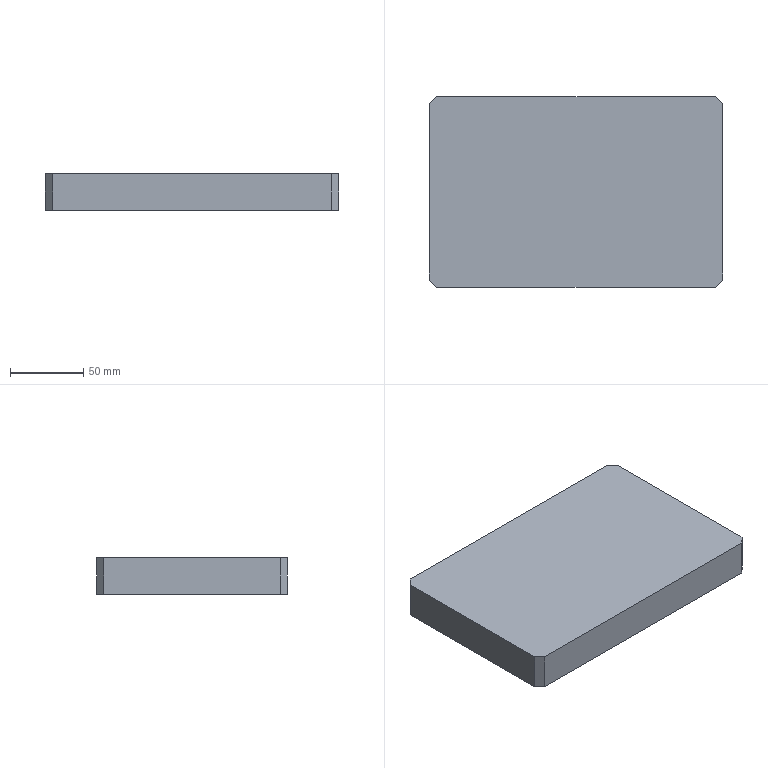Part | SolidWorks | features Chamfer 1, Extrusion 1 | 1 solid | 10 faces | box 200 x 130 x 25 mm | volume 648750 mm3 | plane 10
STEP:
#1=CARTESIAN_POINT('',(100.,-60.,25.));
#2=VERTEX_POINT('',#1);
#3=CARTESIAN_POINT('',(100.,60.,25.));
#4=VERTEX_POINT('',#3);
#5=CARTESIAN_POINT('',(100.,65.,25.));
#6=DIRECTION('',(0.,1.,0.));
#7=VECTOR('',#6,1000.);
#8=LINE('',#5,#7);
#9=EDGE_CURVE('',#2,#4,#8,.T.);
#10=ORIENTED_EDGE('',*,*,#9,.F.);
#11=CARTESIAN_POINT('',(100.,-60.,0.));
#12=VERTEX_POINT('',#11);
#13=CARTESIAN_POINT('',(100.,-60.,25.));
#14=DIRECTION('',(0.,0.,-1.));
#15=VECTOR('',#14,1000.);
#16=LINE('',#13,#15);
#17=EDGE_CURVE('',#2,#12,#16,.T.);
#18=ORIENTED_EDGE('',*,*,#17,.T.);
#19=CARTESIAN_POINT('',(100.,60.,0.));
#20=VERTEX_POINT('',#19);
#21=CARTESIAN_POINT('',(100.,65.,0.));
#22=DIRECTION('',(0.,1.,0.));
#23=VECTOR('',#22,1000.);
#24=LINE('',#21,#23);
#25=EDGE_CURVE('',#12,#20,#24,.T.);
#26=ORIENTED_EDGE('',*,*,#25,.T.);
#27=CARTESIAN_POINT('',(100.,60.,25.));
#28=DIRECTION('',(0.,0.,1.));
#29=VECTOR('',#28,1000.);
#30=LINE('',#27,#29);
#31=EDGE_CURVE('',#20,#4,#30,.T.);
#32=ORIENTED_EDGE('',*,*,#31,.T.);
#33=EDGE_LOOP('',(#10,#18,#26,#32));
#34=FACE_OUTER_BOUND('',#33,.T.);
#35=CARTESIAN_POINT('',(100.,65.,25.));
#36=DIRECTION('',(-1.,0.,0.));
#37=DIRECTION('',(0.,-1.,0.));
#38=AXIS2_PLACEMENT_3D('',#35,#36,#37);
#39=PLANE('',#38);
#40=ADVANCED_FACE('',(#34),#39,.F.);
#41=CARTESIAN_POINT('',(95.,65.,0.));
#42=VERTEX_POINT('',#41);
#43=CARTESIAN_POINT('',(-95.,65.,0.));
#44=VERTEX_POINT('',#43);
#45=CARTESIAN_POINT('',(-100.,65.,0.));
#46=DIRECTION('',(-1.,0.,0.));
#47=VECTOR('',#46,1000.);
#48=LINE('',#45,#47);
#49=EDGE_CURVE('',#42,#44,#48,.T.);
#50=ORIENTED_EDGE('',*,*,#49,.T.);
#51=CARTESIAN_POINT('',(-95.,65.,25.));
#52=VERTEX_POINT('',#51);
#53=CARTESIAN_POINT('',(-95.,65.,25.));
#54=DIRECTION('',(0.,0.,1.));
#55=VECTOR('',#54,1000.);
#56=LINE('',#53,#55);
#57=EDGE_CURVE('',#44,#52,#56,.T.);
#58=ORIENTED_EDGE('',*,*,#57,.T.);
#59=CARTESIAN_POINT('',(95.,65.,25.));
#60=VERTEX_POINT('',#59);
#61=CARTESIAN_POINT('',(-100.,65.,25.));
#62=DIRECTION('',(-1.,0.,0.));
#63=VECTOR('',#62,1000.);
#64=LINE('',#61,#63);
#65=EDGE_CURVE('',#60,#52,#64,.T.);
#66=ORIENTED_EDGE('',*,*,#65,.F.);
#67=CARTESIAN_POINT('',(95.,65.,25.));
#68=DIRECTION('',(0.,0.,-1.));
#69=VECTOR('',#68,1000.);
#70=LINE('',#67,#69);
#71=EDGE_CURVE('',#60,#42,#70,.T.);
#72=ORIENTED_EDGE('',*,*,#71,.T.);
#73=EDGE_LOOP('',(#50,#58,#66,#72));
#74=FACE_OUTER_BOUND('',#73,.T.);
#75=CARTESIAN_POINT('',(-100.,65.,25.));
#76=DIRECTION('',(0.,-1.,0.));
#77=DIRECTION('',(0.,0.,-1.));
#78=AXIS2_PLACEMENT_3D('',#75,#76,#77);
#79=PLANE('',#78);
#80=ADVANCED_FACE('',(#74),#79,.F.);
#81=CARTESIAN_POINT('',(-100.,60.,0.));
#82=VERTEX_POINT('',#81);
#83=CARTESIAN_POINT('',(-100.,-60.,0.));
#84=VERTEX_POINT('',#83);
#85=CARTESIAN_POINT('',(-100.,65.,0.));
#86=DIRECTION('',(0.,-1.,0.));
#87=VECTOR('',#86,1000.);
#88=LINE('',#85,#87);
#89=EDGE_CURVE('',#82,#84,#88,.T.);
#90=ORIENTED_EDGE('',*,*,#89,.T.);
#91=CARTESIAN_POINT('',(-100.,-60.,25.));
#92=VERTEX_POINT('',#91);
#93=CARTESIAN_POINT('',(-100.,-60.,25.));
#94=DIRECTION('',(0.,0.,1.));
#95=VECTOR('',#94,1000.);
#96=LINE('',#93,#95);
#97=EDGE_CURVE('',#84,#92,#96,.T.);
#98=ORIENTED_EDGE('',*,*,#97,.T.);
#99=CARTESIAN_POINT('',(-100.,60.,25.));
#100=VERTEX_POINT('',#99);
#101=CARTESIAN_POINT('',(-100.,65.,25.));
#102=DIRECTION('',(0.,-1.,0.));
#103=VECTOR('',#102,1000.);
#104=LINE('',#101,#103);
#105=EDGE_CURVE('',#100,#92,#104,.T.);
#106=ORIENTED_EDGE('',*,*,#105,.F.);
#107=CARTESIAN_POINT('',(-100.,60.,25.));
#108=DIRECTION('',(0.,0.,-1.));
#109=VECTOR('',#108,1000.);
#110=LINE('',#107,#109);
#111=EDGE_CURVE('',#100,#82,#110,.T.);
#112=ORIENTED_EDGE('',*,*,#111,.T.);
#113=EDGE_LOOP('',(#90,#98,#106,#112));
#114=FACE_OUTER_BOUND('',#113,.T.);
#115=CARTESIAN_POINT('',(-100.,65.,25.));
#116=DIRECTION('',(1.,0.,0.));
#117=DIRECTION('',(0.,1.,0.));
#118=AXIS2_PLACEMENT_3D('',#115,#116,#117);
#119=PLANE('',#118);
#120=ADVANCED_FACE('',(#114),#119,.F.);
#121=CARTESIAN_POINT('',(-95.,-65.,25.));
#122=VERTEX_POINT('',#121);
#123=CARTESIAN_POINT('',(95.,-65.,25.));
#124=VERTEX_POINT('',#123);
#125=CARTESIAN_POINT('',(-100.,-65.,25.));
#126=DIRECTION('',(1.,0.,0.));
#127=VECTOR('',#126,1000.);
#128=LINE('',#125,#127);
#129=EDGE_CURVE('',#122,#124,#128,.T.);
#130=ORIENTED_EDGE('',*,*,#129,.F.);
#131=CARTESIAN_POINT('',(-95.,-65.,0.));
#132=VERTEX_POINT('',#131);
#133=CARTESIAN_POINT('',(-95.,-65.,25.));
#134=DIRECTION('',(0.,0.,-1.));
#135=VECTOR('',#134,1000.);
#136=LINE('',#133,#135);
#137=EDGE_CURVE('',#122,#132,#136,.T.);
#138=ORIENTED_EDGE('',*,*,#137,.T.);
#139=CARTESIAN_POINT('',(95.,-65.,0.));
#140=VERTEX_POINT('',#139);
#141=CARTESIAN_POINT('',(-100.,-65.,0.));
#142=DIRECTION('',(1.,0.,0.));
#143=VECTOR('',#142,1000.);
#144=LINE('',#141,#143);
#145=EDGE_CURVE('',#132,#140,#144,.T.);
#146=ORIENTED_EDGE('',*,*,#145,.T.);
#147=CARTESIAN_POINT('',(95.,-65.,25.));
#148=DIRECTION('',(0.,0.,1.));
#149=VECTOR('',#148,1000.);
#150=LINE('',#147,#149);
#151=EDGE_CURVE('',#140,#124,#150,.T.);
#152=ORIENTED_EDGE('',*,*,#151,.T.);
#153=EDGE_LOOP('',(#130,#138,#146,#152));
#154=FACE_OUTER_BOUND('',#153,.T.);
#155=CARTESIAN_POINT('',(-100.,-65.,25.));
#156=DIRECTION('',(0.,1.,0.));
#157=DIRECTION('',(0.,0.,1.));
#158=AXIS2_PLACEMENT_3D('',#155,#156,#157);
#159=PLANE('',#158);
#160=ADVANCED_FACE('',(#154),#159,.F.);
#161=ORIENTED_EDGE('',*,*,#105,.T.);
#162=CARTESIAN_POINT('',(-80.,-80.,25.));
#163=DIRECTION('',(0.7071,-0.7071,0.));
#164=VECTOR('',#163,1000.);
#165=LINE('',#162,#164);
#166=EDGE_CURVE('',#92,#122,#165,.T.);
#167=ORIENTED_EDGE('',*,*,#166,.T.);
#168=ORIENTED_EDGE('',*,*,#129,.T.);
#169=CARTESIAN_POINT('',(80.,-80.,25.));
#170=DIRECTION('',(0.7071,0.7071,0.));
#171=VECTOR('',#170,1000.);
#172=LINE('',#169,#171);
#173=EDGE_CURVE('',#124,#2,#172,.T.);
#174=ORIENTED_EDGE('',*,*,#173,.T.);
#175=ORIENTED_EDGE('',*,*,#9,.T.);
#176=CARTESIAN_POINT('',(80.,80.,25.));
#177=DIRECTION('',(-0.7071,0.7071,0.));
#178=VECTOR('',#177,1000.);
#179=LINE('',#176,#178);
#180=EDGE_CURVE('',#4,#60,#179,.T.);
#181=ORIENTED_EDGE('',*,*,#180,.T.);
#182=ORIENTED_EDGE('',*,*,#65,.T.);
#183=CARTESIAN_POINT('',(-80.,80.,25.));
#184=DIRECTION('',(-0.7071,-0.7071,0.));
#185=VECTOR('',#184,1000.);
#186=LINE('',#183,#185);
#187=EDGE_CURVE('',#52,#100,#186,.T.);
#188=ORIENTED_EDGE('',*,*,#187,.T.);
#189=EDGE_LOOP('',(#161,#167,#168,#174,#175,#181,#182,#188));
#190=FACE_OUTER_BOUND('',#189,.T.);
#191=CARTESIAN_POINT('',(0.,0.,25.));
#192=DIRECTION('',(0.,0.,1.));
#193=DIRECTION('',(1.,0.,0.));
#194=AXIS2_PLACEMENT_3D('',#191,#192,#193);
#195=PLANE('',#194);
#196=ADVANCED_FACE('',(#190),#195,.T.);
#197=ORIENTED_EDGE('',*,*,#145,.F.);
#198=CARTESIAN_POINT('',(-95.,-65.,0.));
#199=DIRECTION('',(-0.7071,0.7071,0.));
#200=VECTOR('',#199,1000.);
#201=LINE('',#198,#200);
#202=EDGE_CURVE('',#132,#84,#201,.T.);
#203=ORIENTED_EDGE('',*,*,#202,.T.);
#204=ORIENTED_EDGE('',*,*,#89,.F.);
#205=CARTESIAN_POINT('',(-100.,60.,0.));
#206=DIRECTION('',(0.7071,0.7071,0.));
#207=VECTOR('',#206,1000.);
#208=LINE('',#205,#207);
#209=EDGE_CURVE('',#82,#44,#208,.T.);
#210=ORIENTED_EDGE('',*,*,#209,.T.);
#211=ORIENTED_EDGE('',*,*,#49,.F.);
#212=CARTESIAN_POINT('',(95.,65.,0.));
#213=DIRECTION('',(0.7071,-0.7071,0.));
#214=VECTOR('',#213,1000.);
#215=LINE('',#212,#214);
#216=EDGE_CURVE('',#42,#20,#215,.T.);
#217=ORIENTED_EDGE('',*,*,#216,.T.);
#218=ORIENTED_EDGE('',*,*,#25,.F.);
#219=CARTESIAN_POINT('',(100.,-60.,0.));
#220=DIRECTION('',(-0.7071,-0.7071,0.));
#221=VECTOR('',#220,1000.);
#222=LINE('',#219,#221);
#223=EDGE_CURVE('',#12,#140,#222,.T.);
#224=ORIENTED_EDGE('',*,*,#223,.T.);
#225=EDGE_LOOP('',(#197,#203,#204,#210,#211,#217,#218,#224));
#226=FACE_OUTER_BOUND('',#225,.T.);
#227=CARTESIAN_POINT('',(0.,0.,0.));
#228=DIRECTION('',(0.,0.,1.));
#229=DIRECTION('',(1.,0.,0.));
#230=AXIS2_PLACEMENT_3D('',#227,#228,#229);
#231=PLANE('',#230);
#232=ADVANCED_FACE('',(#226),#231,.F.);
#233=ORIENTED_EDGE('',*,*,#166,.F.);
#234=ORIENTED_EDGE('',*,*,#97,.F.);
#235=ORIENTED_EDGE('',*,*,#202,.F.);
#236=ORIENTED_EDGE('',*,*,#137,.F.);
#237=EDGE_LOOP('',(#233,#234,#235,#236));
#238=FACE_OUTER_BOUND('',#237,.T.);
#239=CARTESIAN_POINT('',(-95.,-65.,25.));
#240=DIRECTION('',(0.7071,0.7071,0.));
#241=DIRECTION('',(0.,0.,-1.));
#242=AXIS2_PLACEMENT_3D('',#239,#240,#241);
#243=PLANE('',#242);
#244=ADVANCED_FACE('',(#238),#243,.F.);
#245=ORIENTED_EDGE('',*,*,#173,.F.);
#246=ORIENTED_EDGE('',*,*,#151,.F.);
#247=ORIENTED_EDGE('',*,*,#223,.F.);
#248=ORIENTED_EDGE('',*,*,#17,.F.);
#249=EDGE_LOOP('',(#245,#246,#247,#248));
#250=FACE_OUTER_BOUND('',#249,.T.);
#251=CARTESIAN_POINT('',(100.,-60.,25.));
#252=DIRECTION('',(-0.7071,0.7071,0.));
#253=DIRECTION('',(0.,0.,-1.));
#254=AXIS2_PLACEMENT_3D('',#251,#252,#253);
#255=PLANE('',#254);
#256=ADVANCED_FACE('',(#250),#255,.F.);
#257=ORIENTED_EDGE('',*,*,#187,.F.);
#258=ORIENTED_EDGE('',*,*,#57,.F.);
#259=ORIENTED_EDGE('',*,*,#209,.F.);
#260=ORIENTED_EDGE('',*,*,#111,.F.);
#261=EDGE_LOOP('',(#257,#258,#259,#260));
#262=FACE_OUTER_BOUND('',#261,.T.);
#263=CARTESIAN_POINT('',(-100.,60.,25.));
#264=DIRECTION('',(0.7071,-0.7071,0.));
#265=DIRECTION('',(0.,0.,-1.));
#266=AXIS2_PLACEMENT_3D('',#263,#264,#265);
#267=PLANE('',#266);
#268=ADVANCED_FACE('',(#262),#267,.F.);
#269=ORIENTED_EDGE('',*,*,#180,.F.);
#270=ORIENTED_EDGE('',*,*,#31,.F.);
#271=ORIENTED_EDGE('',*,*,#216,.F.);
#272=ORIENTED_EDGE('',*,*,#71,.F.);
#273=EDGE_LOOP('',(#269,#270,#271,#272));
#274=FACE_OUTER_BOUND('',#273,.T.);
#275=CARTESIAN_POINT('',(95.,65.,25.));
#276=DIRECTION('',(-0.7071,-0.7071,0.));
#277=DIRECTION('',(0.,0.,-1.));
#278=AXIS2_PLACEMENT_3D('',#275,#276,#277);
#279=PLANE('',#278);
#280=ADVANCED_FACE('',(#274),#279,.F.);
#281=CLOSED_SHELL('',(#40,#80,#120,#160,#196,#232,#244,#256,#268,#280));
#282=MANIFOLD_SOLID_BREP('',#281);
#283=CARTESIAN_POINT('',(0.,0.,0.));
#284=DIRECTION('',(0.,0.,1.));
#285=DIRECTION('',(1.,0.,0.));
#286=AXIS2_PLACEMENT_3D('',#283,#284,#285);
#287=(LENGTH_UNIT()NAMED_UNIT(*)SI_UNIT(.MILLI.,.METRE.));
#288=UNCERTAINTY_MEASURE_WITH_UNIT(LENGTH_MEASURE(0.00001),#287,'','');
#289=(NAMED_UNIT(*)PLANE_ANGLE_UNIT()SI_UNIT($,.RADIAN.));
#290=(NAMED_UNIT(*)SI_UNIT($,.STERADIAN.)SOLID_ANGLE_UNIT());
#291=(GEOMETRIC_REPRESENTATION_CONTEXT(3)GLOBAL_UNCERTAINTY_ASSIGNED_CONTEXT((#288))GLOBAL_UNIT_ASSIGNED_CONTEXT((#287,#289,#290))REPRESENTATION_CONTEXT('',''));
#292=ADVANCED_BREP_SHAPE_REPRESENTATION('',(#282,#286),#291);